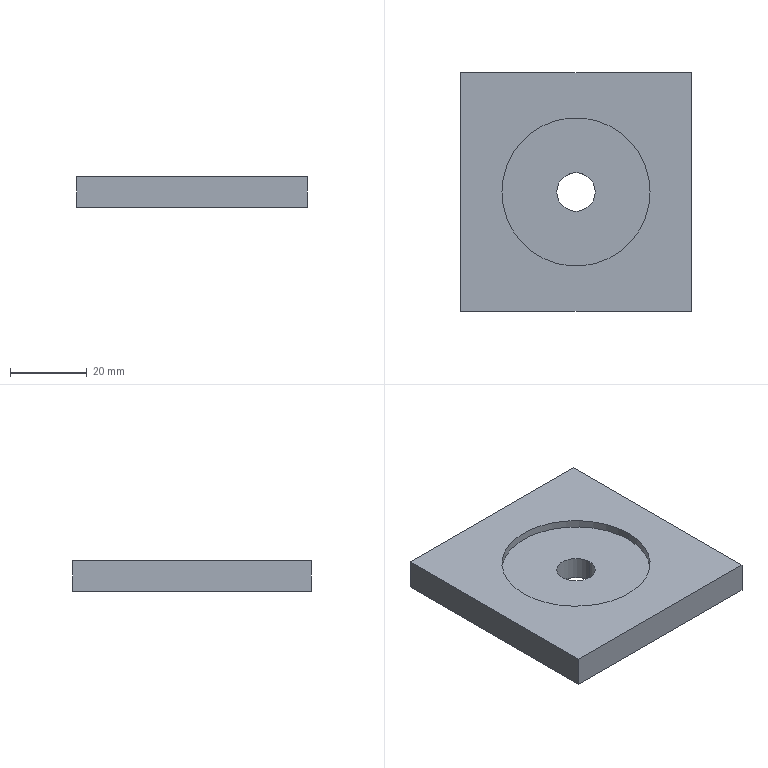Part | SolidWorks | features Cut 2, Extrusion 1 | 1 solid | 11 faces | box 60 x 62 x 8 mm | volume 26960 mm3 | plane 7 | cylinder 4 | commonest cylinder face diameters 10 x2 38.5 x2
STEP:
#1=CARTESIAN_POINT('',(-5.,0.,0.));
#2=VERTEX_POINT('',#1);
#3=CARTESIAN_POINT('',(5.,0.,0.));
#4=VERTEX_POINT('',#3);
#5=CARTESIAN_POINT('',(0.,0.,0.));
#6=DIRECTION('',(0.,0.,1.));
#7=DIRECTION('',(1.,0.,0.));
#8=AXIS2_PLACEMENT_3D('',#5,#6,#7);
#9=CIRCLE('',#8,5.);
#10=EDGE_CURVE('',#2,#4,#9,.T.);
#11=ORIENTED_EDGE('',*,*,#10,.F.);
#12=CARTESIAN_POINT('',(-5.,0.,6.));
#13=VERTEX_POINT('',#12);
#14=CARTESIAN_POINT('',(-5.,0.,0.));
#15=DIRECTION('',(0.,0.,1.));
#16=VECTOR('',#15,1000.);
#17=LINE('',#14,#16);
#18=EDGE_CURVE('',#2,#13,#17,.T.);
#19=ORIENTED_EDGE('',*,*,#18,.T.);
#20=CARTESIAN_POINT('',(5.,0.,6.));
#21=VERTEX_POINT('',#20);
#22=CARTESIAN_POINT('',(0.,0.,6.));
#23=DIRECTION('',(0.,0.,1.));
#24=DIRECTION('',(1.,0.,0.));
#25=AXIS2_PLACEMENT_3D('',#22,#23,#24);
#26=CIRCLE('',#25,5.);
#27=EDGE_CURVE('',#13,#21,#26,.T.);
#28=ORIENTED_EDGE('',*,*,#27,.T.);
#29=CARTESIAN_POINT('',(5.,0.,0.));
#30=DIRECTION('',(0.,0.,1.));
#31=VECTOR('',#30,1000.);
#32=LINE('',#29,#31);
#33=EDGE_CURVE('',#4,#21,#32,.T.);
#34=ORIENTED_EDGE('',*,*,#33,.F.);
#35=EDGE_LOOP('',(#11,#19,#28,#34));
#36=FACE_OUTER_BOUND('',#35,.T.);
#37=CARTESIAN_POINT('',(0.,0.,0.));
#38=DIRECTION('',(0.,0.,1.));
#39=DIRECTION('',(1.,0.,0.));
#40=AXIS2_PLACEMENT_3D('',#37,#38,#39);
#41=CYLINDRICAL_SURFACE('',#40,5.);
#42=ADVANCED_FACE('',(#36),#41,.F.);
#43=CARTESIAN_POINT('',(-19.25,0.,6.));
#44=VERTEX_POINT('',#43);
#45=CARTESIAN_POINT('',(19.25,0.,6.));
#46=VERTEX_POINT('',#45);
#47=CARTESIAN_POINT('',(0.,0.,6.));
#48=DIRECTION('',(0.,0.,1.));
#49=DIRECTION('',(1.,0.,0.));
#50=AXIS2_PLACEMENT_3D('',#47,#48,#49);
#51=CIRCLE('',#50,19.25);
#52=EDGE_CURVE('',#44,#46,#51,.T.);
#53=ORIENTED_EDGE('',*,*,#52,.F.);
#54=CARTESIAN_POINT('',(-19.25,0.,8.));
#55=VERTEX_POINT('',#54);
#56=CARTESIAN_POINT('',(-19.25,0.,6.));
#57=DIRECTION('',(0.,0.,1.));
#58=VECTOR('',#57,1000.);
#59=LINE('',#56,#58);
#60=EDGE_CURVE('',#44,#55,#59,.T.);
#61=ORIENTED_EDGE('',*,*,#60,.T.);
#62=CARTESIAN_POINT('',(19.25,0.,8.));
#63=VERTEX_POINT('',#62);
#64=CARTESIAN_POINT('',(0.,0.,8.));
#65=DIRECTION('',(0.,0.,1.));
#66=DIRECTION('',(1.,0.,0.));
#67=AXIS2_PLACEMENT_3D('',#64,#65,#66);
#68=CIRCLE('',#67,19.25);
#69=EDGE_CURVE('',#55,#63,#68,.T.);
#70=ORIENTED_EDGE('',*,*,#69,.T.);
#71=CARTESIAN_POINT('',(19.25,0.,6.));
#72=DIRECTION('',(0.,0.,1.));
#73=VECTOR('',#72,1000.);
#74=LINE('',#71,#73);
#75=EDGE_CURVE('',#46,#63,#74,.T.);
#76=ORIENTED_EDGE('',*,*,#75,.F.);
#77=EDGE_LOOP('',(#53,#61,#70,#76));
#78=FACE_OUTER_BOUND('',#77,.T.);
#79=CARTESIAN_POINT('',(0.,0.,6.));
#80=DIRECTION('',(0.,0.,1.));
#81=DIRECTION('',(1.,0.,0.));
#82=AXIS2_PLACEMENT_3D('',#79,#80,#81);
#83=CYLINDRICAL_SURFACE('',#82,19.25);
#84=ADVANCED_FACE('',(#78),#83,.F.);
#85=CARTESIAN_POINT('',(30.,-31.,0.));
#86=VERTEX_POINT('',#85);
#87=CARTESIAN_POINT('',(30.,31.,0.));
#88=VERTEX_POINT('',#87);
#89=CARTESIAN_POINT('',(30.,31.,0.));
#90=DIRECTION('',(0.,1.,0.));
#91=VECTOR('',#90,1000.);
#92=LINE('',#89,#91);
#93=EDGE_CURVE('',#86,#88,#92,.T.);
#94=ORIENTED_EDGE('',*,*,#93,.T.);
#95=CARTESIAN_POINT('',(30.,31.,8.));
#96=VERTEX_POINT('',#95);
#97=CARTESIAN_POINT('',(30.,31.,8.));
#98=DIRECTION('',(0.,0.,-1.));
#99=VECTOR('',#98,1000.);
#100=LINE('',#97,#99);
#101=EDGE_CURVE('',#96,#88,#100,.T.);
#102=ORIENTED_EDGE('',*,*,#101,.F.);
#103=CARTESIAN_POINT('',(30.,-31.,8.));
#104=VERTEX_POINT('',#103);
#105=CARTESIAN_POINT('',(30.,31.,8.));
#106=DIRECTION('',(0.,1.,0.));
#107=VECTOR('',#106,1000.);
#108=LINE('',#105,#107);
#109=EDGE_CURVE('',#104,#96,#108,.T.);
#110=ORIENTED_EDGE('',*,*,#109,.F.);
#111=CARTESIAN_POINT('',(30.,-31.,8.));
#112=DIRECTION('',(0.,0.,-1.));
#113=VECTOR('',#112,1000.);
#114=LINE('',#111,#113);
#115=EDGE_CURVE('',#104,#86,#114,.T.);
#116=ORIENTED_EDGE('',*,*,#115,.T.);
#117=EDGE_LOOP('',(#94,#102,#110,#116));
#118=FACE_OUTER_BOUND('',#117,.T.);
#119=CARTESIAN_POINT('',(30.,31.,8.));
#120=DIRECTION('',(-1.,0.,0.));
#121=DIRECTION('',(0.,-1.,0.));
#122=AXIS2_PLACEMENT_3D('',#119,#120,#121);
#123=PLANE('',#122);
#124=ADVANCED_FACE('',(#118),#123,.F.);
#125=CARTESIAN_POINT('',(-30.,31.,0.));
#126=VERTEX_POINT('',#125);
#127=CARTESIAN_POINT('',(-30.,31.,0.));
#128=DIRECTION('',(-1.,0.,0.));
#129=VECTOR('',#128,1000.);
#130=LINE('',#127,#129);
#131=EDGE_CURVE('',#88,#126,#130,.T.);
#132=ORIENTED_EDGE('',*,*,#131,.T.);
#133=CARTESIAN_POINT('',(-30.,31.,8.));
#134=VERTEX_POINT('',#133);
#135=CARTESIAN_POINT('',(-30.,31.,8.));
#136=DIRECTION('',(0.,0.,-1.));
#137=VECTOR('',#136,1000.);
#138=LINE('',#135,#137);
#139=EDGE_CURVE('',#134,#126,#138,.T.);
#140=ORIENTED_EDGE('',*,*,#139,.F.);
#141=CARTESIAN_POINT('',(-30.,31.,8.));
#142=DIRECTION('',(-1.,0.,0.));
#143=VECTOR('',#142,1000.);
#144=LINE('',#141,#143);
#145=EDGE_CURVE('',#96,#134,#144,.T.);
#146=ORIENTED_EDGE('',*,*,#145,.F.);
#147=ORIENTED_EDGE('',*,*,#101,.T.);
#148=EDGE_LOOP('',(#132,#140,#146,#147));
#149=FACE_OUTER_BOUND('',#148,.T.);
#150=CARTESIAN_POINT('',(-30.,31.,8.));
#151=DIRECTION('',(0.,-1.,0.));
#152=DIRECTION('',(0.,0.,-1.));
#153=AXIS2_PLACEMENT_3D('',#150,#151,#152);
#154=PLANE('',#153);
#155=ADVANCED_FACE('',(#149),#154,.F.);
#156=CARTESIAN_POINT('',(-30.,-31.,0.));
#157=VERTEX_POINT('',#156);
#158=CARTESIAN_POINT('',(-30.,31.,0.));
#159=DIRECTION('',(0.,-1.,0.));
#160=VECTOR('',#159,1000.);
#161=LINE('',#158,#160);
#162=EDGE_CURVE('',#126,#157,#161,.T.);
#163=ORIENTED_EDGE('',*,*,#162,.T.);
#164=CARTESIAN_POINT('',(-30.,-31.,8.));
#165=VERTEX_POINT('',#164);
#166=CARTESIAN_POINT('',(-30.,-31.,8.));
#167=DIRECTION('',(0.,0.,-1.));
#168=VECTOR('',#167,1000.);
#169=LINE('',#166,#168);
#170=EDGE_CURVE('',#165,#157,#169,.T.);
#171=ORIENTED_EDGE('',*,*,#170,.F.);
#172=CARTESIAN_POINT('',(-30.,31.,8.));
#173=DIRECTION('',(0.,-1.,0.));
#174=VECTOR('',#173,1000.);
#175=LINE('',#172,#174);
#176=EDGE_CURVE('',#134,#165,#175,.T.);
#177=ORIENTED_EDGE('',*,*,#176,.F.);
#178=ORIENTED_EDGE('',*,*,#139,.T.);
#179=EDGE_LOOP('',(#163,#171,#177,#178));
#180=FACE_OUTER_BOUND('',#179,.T.);
#181=CARTESIAN_POINT('',(-30.,31.,8.));
#182=DIRECTION('',(1.,0.,0.));
#183=DIRECTION('',(0.,1.,0.));
#184=AXIS2_PLACEMENT_3D('',#181,#182,#183);
#185=PLANE('',#184);
#186=ADVANCED_FACE('',(#180),#185,.F.);
#187=CARTESIAN_POINT('',(-30.,-31.,0.));
#188=DIRECTION('',(1.,0.,0.));
#189=VECTOR('',#188,1000.);
#190=LINE('',#187,#189);
#191=EDGE_CURVE('',#157,#86,#190,.T.);
#192=ORIENTED_EDGE('',*,*,#191,.T.);
#193=ORIENTED_EDGE('',*,*,#115,.F.);
#194=CARTESIAN_POINT('',(-30.,-31.,8.));
#195=DIRECTION('',(1.,0.,0.));
#196=VECTOR('',#195,1000.);
#197=LINE('',#194,#196);
#198=EDGE_CURVE('',#165,#104,#197,.T.);
#199=ORIENTED_EDGE('',*,*,#198,.F.);
#200=ORIENTED_EDGE('',*,*,#170,.T.);
#201=EDGE_LOOP('',(#192,#193,#199,#200));
#202=FACE_OUTER_BOUND('',#201,.T.);
#203=CARTESIAN_POINT('',(-30.,-31.,8.));
#204=DIRECTION('',(0.,1.,0.));
#205=DIRECTION('',(0.,0.,1.));
#206=AXIS2_PLACEMENT_3D('',#203,#204,#205);
#207=PLANE('',#206);
#208=ADVANCED_FACE('',(#202),#207,.F.);
#209=CARTESIAN_POINT('',(0.,0.,8.));
#210=DIRECTION('',(0.,0.,1.));
#211=DIRECTION('',(1.,0.,0.));
#212=AXIS2_PLACEMENT_3D('',#209,#210,#211);
#213=CIRCLE('',#212,19.25);
#214=EDGE_CURVE('',#63,#55,#213,.T.);
#215=ORIENTED_EDGE('',*,*,#214,.F.);
#216=ORIENTED_EDGE('',*,*,#69,.F.);
#217=EDGE_LOOP('',(#215,#216));
#218=FACE_BOUND('',#217,.T.);
#219=ORIENTED_EDGE('',*,*,#109,.T.);
#220=ORIENTED_EDGE('',*,*,#145,.T.);
#221=ORIENTED_EDGE('',*,*,#176,.T.);
#222=ORIENTED_EDGE('',*,*,#198,.T.);
#223=EDGE_LOOP('',(#219,#220,#221,#222));
#224=FACE_OUTER_BOUND('',#223,.T.);
#225=CARTESIAN_POINT('',(0.,0.,8.));
#226=DIRECTION('',(0.,0.,1.));
#227=DIRECTION('',(1.,0.,0.));
#228=AXIS2_PLACEMENT_3D('',#225,#226,#227);
#229=PLANE('',#228);
#230=ADVANCED_FACE('',(#218,#224),#229,.T.);
#231=CARTESIAN_POINT('',(0.,0.,0.));
#232=DIRECTION('',(0.,0.,1.));
#233=DIRECTION('',(1.,0.,0.));
#234=AXIS2_PLACEMENT_3D('',#231,#232,#233);
#235=CIRCLE('',#234,5.);
#236=EDGE_CURVE('',#4,#2,#235,.T.);
#237=ORIENTED_EDGE('',*,*,#236,.T.);
#238=ORIENTED_EDGE('',*,*,#10,.T.);
#239=EDGE_LOOP('',(#237,#238));
#240=FACE_BOUND('',#239,.T.);
#241=ORIENTED_EDGE('',*,*,#93,.F.);
#242=ORIENTED_EDGE('',*,*,#191,.F.);
#243=ORIENTED_EDGE('',*,*,#162,.F.);
#244=ORIENTED_EDGE('',*,*,#131,.F.);
#245=EDGE_LOOP('',(#241,#242,#243,#244));
#246=FACE_OUTER_BOUND('',#245,.T.);
#247=CARTESIAN_POINT('',(0.,0.,0.));
#248=DIRECTION('',(0.,0.,1.));
#249=DIRECTION('',(1.,0.,0.));
#250=AXIS2_PLACEMENT_3D('',#247,#248,#249);
#251=PLANE('',#250);
#252=ADVANCED_FACE('',(#240,#246),#251,.F.);
#253=ORIENTED_EDGE('',*,*,#60,.F.);
#254=CARTESIAN_POINT('',(0.,0.,6.));
#255=DIRECTION('',(0.,0.,1.));
#256=DIRECTION('',(1.,0.,0.));
#257=AXIS2_PLACEMENT_3D('',#254,#255,#256);
#258=CIRCLE('',#257,19.25);
#259=EDGE_CURVE('',#46,#44,#258,.T.);
#260=ORIENTED_EDGE('',*,*,#259,.F.);
#261=ORIENTED_EDGE('',*,*,#75,.T.);
#262=ORIENTED_EDGE('',*,*,#214,.T.);
#263=EDGE_LOOP('',(#253,#260,#261,#262));
#264=FACE_OUTER_BOUND('',#263,.T.);
#265=CARTESIAN_POINT('',(0.,0.,6.));
#266=DIRECTION('',(0.,0.,1.));
#267=DIRECTION('',(1.,0.,0.));
#268=AXIS2_PLACEMENT_3D('',#265,#266,#267);
#269=CYLINDRICAL_SURFACE('',#268,19.25);
#270=ADVANCED_FACE('',(#264),#269,.F.);
#271=CARTESIAN_POINT('',(0.,0.,6.));
#272=DIRECTION('',(0.,0.,1.));
#273=DIRECTION('',(1.,0.,0.));
#274=AXIS2_PLACEMENT_3D('',#271,#272,#273);
#275=CIRCLE('',#274,5.);
#276=EDGE_CURVE('',#21,#13,#275,.T.);
#277=ORIENTED_EDGE('',*,*,#276,.F.);
#278=ORIENTED_EDGE('',*,*,#27,.F.);
#279=EDGE_LOOP('',(#277,#278));
#280=FACE_BOUND('',#279,.T.);
#281=ORIENTED_EDGE('',*,*,#259,.T.);
#282=ORIENTED_EDGE('',*,*,#52,.T.);
#283=EDGE_LOOP('',(#281,#282));
#284=FACE_OUTER_BOUND('',#283,.T.);
#285=CARTESIAN_POINT('',(0.,0.,6.));
#286=DIRECTION('',(0.,0.,1.));
#287=DIRECTION('',(1.,0.,0.));
#288=AXIS2_PLACEMENT_3D('',#285,#286,#287);
#289=PLANE('',#288);
#290=ADVANCED_FACE('',(#280,#284),#289,.T.);
#291=ORIENTED_EDGE('',*,*,#18,.F.);
#292=ORIENTED_EDGE('',*,*,#236,.F.);
#293=ORIENTED_EDGE('',*,*,#33,.T.);
#294=ORIENTED_EDGE('',*,*,#276,.T.);
#295=EDGE_LOOP('',(#291,#292,#293,#294));
#296=FACE_OUTER_BOUND('',#295,.T.);
#297=CARTESIAN_POINT('',(0.,0.,0.));
#298=DIRECTION('',(0.,0.,1.));
#299=DIRECTION('',(1.,0.,0.));
#300=AXIS2_PLACEMENT_3D('',#297,#298,#299);
#301=CYLINDRICAL_SURFACE('',#300,5.);
#302=ADVANCED_FACE('',(#296),#301,.F.);
#303=CLOSED_SHELL('',(#42,#84,#124,#155,#186,#208,#230,#252,#270,#290,#302));
#304=MANIFOLD_SOLID_BREP('',#303);
#305=CARTESIAN_POINT('',(0.,0.,0.));
#306=DIRECTION('',(0.,0.,1.));
#307=DIRECTION('',(1.,0.,0.));
#308=AXIS2_PLACEMENT_3D('',#305,#306,#307);
#309=(LENGTH_UNIT()NAMED_UNIT(*)SI_UNIT(.MILLI.,.METRE.));
#310=UNCERTAINTY_MEASURE_WITH_UNIT(LENGTH_MEASURE(0.00001),#309,'','');
#311=(NAMED_UNIT(*)PLANE_ANGLE_UNIT()SI_UNIT($,.RADIAN.));
#312=(NAMED_UNIT(*)SI_UNIT($,.STERADIAN.)SOLID_ANGLE_UNIT());
#313=(GEOMETRIC_REPRESENTATION_CONTEXT(3)GLOBAL_UNCERTAINTY_ASSIGNED_CONTEXT((#310))GLOBAL_UNIT_ASSIGNED_CONTEXT((#309,#311,#312))REPRESENTATION_CONTEXT('',''));
#314=ADVANCED_BREP_SHAPE_REPRESENTATION('',(#304,#308),#313);